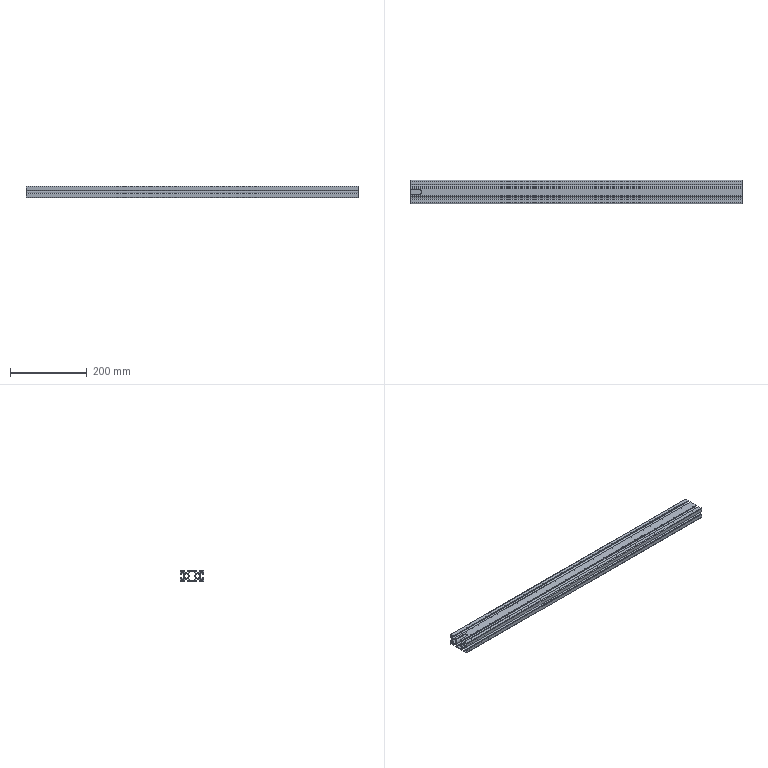Part | STEP file | 1 solid | 161 faces | box 865 x 60 x 30 mm | volume 559855 mm3 | plane 85 | cylinder 68 | cone 8 | commonest cylinder face diameters 2 x26 16 x14 1 x10 12 x8 3 x4 11.5 x4